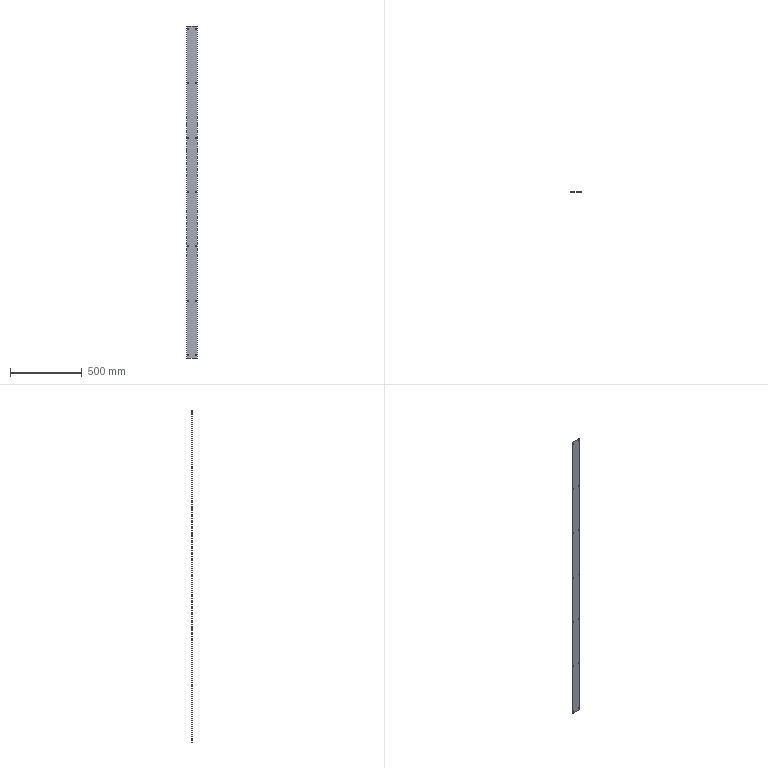Part | 1 solid | 62 faces | box 70 x 1 x 2316 mm | volume 161472 mm3 | plane 34 | cylinder 28 | commonest cylinder face diameters 6 x28